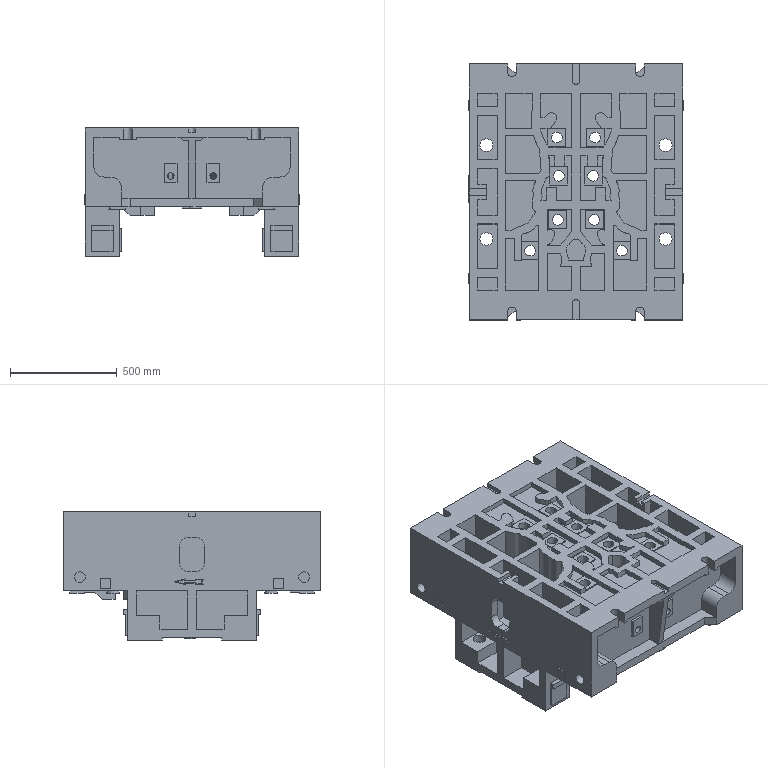Part | NX | features solid 2 | 1 solid | 855 faces | box 1010 x 1200 x 600 mm | volume 211034440 mm3 | plane 717 | cylinder 106 | spline 32 | commonest cylinder face diameters 60 x16 50 x14 80 x14 30 x12 50.5 x8 100 x8